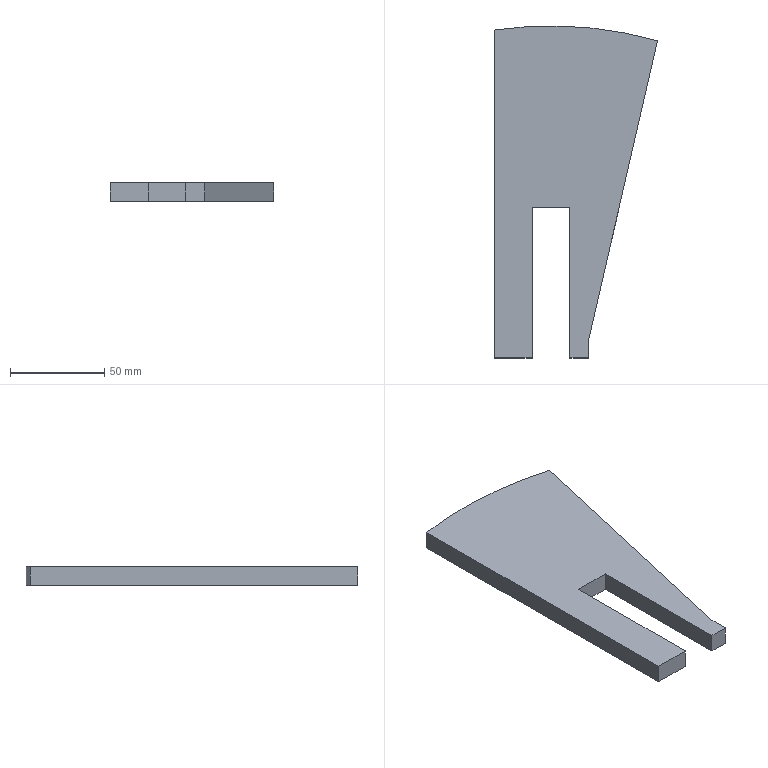Part | SolidWorks | features Extrusion 1, ICE 1 | 1 solid | 11 faces | box 86.5 x 176 x 10 mm | volume 102042 mm3 | plane 10 | cylinder 1 | commonest cylinder face diameters 412 x1
STEP:
#1=CARTESIAN_POINT('',(-30.,30.,-5.));
#2=VERTEX_POINT('',#1);
#3=CARTESIAN_POINT('',(-10.,30.,-5.));
#4=VERTEX_POINT('',#3);
#5=CARTESIAN_POINT('',(20.,30.,-5.));
#6=DIRECTION('',(1.,0.,0.));
#7=VECTOR('',#6,1000.);
#8=LINE('',#5,#7);
#9=EDGE_CURVE('',#2,#4,#8,.T.);
#10=ORIENTED_EDGE('',*,*,#9,.T.);
#11=CARTESIAN_POINT('',(-10.,30.,5.));
#12=VERTEX_POINT('',#11);
#13=CARTESIAN_POINT('',(-10.,30.,5.));
#14=DIRECTION('',(0.,0.,1.));
#15=VECTOR('',#14,1000.);
#16=LINE('',#13,#15);
#17=EDGE_CURVE('',#4,#12,#16,.T.);
#18=ORIENTED_EDGE('',*,*,#17,.T.);
#19=CARTESIAN_POINT('',(-30.,30.,5.));
#20=VERTEX_POINT('',#19);
#21=CARTESIAN_POINT('',(20.,30.,5.));
#22=DIRECTION('',(1.,0.,0.));
#23=VECTOR('',#22,1000.);
#24=LINE('',#21,#23);
#25=EDGE_CURVE('',#20,#12,#24,.T.);
#26=ORIENTED_EDGE('',*,*,#25,.F.);
#27=CARTESIAN_POINT('',(-30.,30.,5.));
#28=DIRECTION('',(0.,0.,-1.));
#29=VECTOR('',#28,1000.);
#30=LINE('',#27,#29);
#31=EDGE_CURVE('',#20,#2,#30,.T.);
#32=ORIENTED_EDGE('',*,*,#31,.T.);
#33=EDGE_LOOP('',(#10,#18,#26,#32));
#34=FACE_OUTER_BOUND('',#33,.T.);
#35=CARTESIAN_POINT('',(20.,30.,5.));
#36=DIRECTION('',(0.,1.,0.));
#37=DIRECTION('',(-1.,0.,0.));
#38=AXIS2_PLACEMENT_3D('',#35,#36,#37);
#39=PLANE('',#38);
#40=ADVANCED_FACE('',(#34),#39,.F.);
#41=CARTESIAN_POINT('',(56.5,198.1,-5.));
#42=VERTEX_POINT('',#41);
#43=CARTESIAN_POINT('',(-30.,203.804,-5.));
#44=VERTEX_POINT('',#43);
#45=CARTESIAN_POINT('',(0.,0.,-5.));
#46=DIRECTION('',(0.,0.,1.));
#47=DIRECTION('',(1.,0.,0.));
#48=AXIS2_PLACEMENT_3D('',#45,#46,#47);
#49=CIRCLE('',#48,206.);
#50=EDGE_CURVE('',#42,#44,#49,.T.);
#51=ORIENTED_EDGE('',*,*,#50,.T.);
#52=CARTESIAN_POINT('',(-30.,203.804,5.));
#53=VERTEX_POINT('',#52);
#54=CARTESIAN_POINT('',(-30.,203.804,5.));
#55=DIRECTION('',(0.,0.,-1.));
#56=VECTOR('',#55,1000.);
#57=LINE('',#54,#56);
#58=EDGE_CURVE('',#53,#44,#57,.T.);
#59=ORIENTED_EDGE('',*,*,#58,.F.);
#60=CARTESIAN_POINT('',(56.5,198.1,5.));
#61=VERTEX_POINT('',#60);
#62=CARTESIAN_POINT('',(0.,0.,5.));
#63=DIRECTION('',(0.,0.,1.));
#64=DIRECTION('',(1.,0.,0.));
#65=AXIS2_PLACEMENT_3D('',#62,#63,#64);
#66=CIRCLE('',#65,206.);
#67=EDGE_CURVE('',#61,#53,#66,.T.);
#68=ORIENTED_EDGE('',*,*,#67,.F.);
#69=CARTESIAN_POINT('',(56.5,198.1,5.));
#70=DIRECTION('',(0.,0.,-1.));
#71=VECTOR('',#70,1000.);
#72=LINE('',#69,#71);
#73=EDGE_CURVE('',#61,#42,#72,.T.);
#74=ORIENTED_EDGE('',*,*,#73,.T.);
#75=EDGE_LOOP('',(#51,#59,#68,#74));
#76=FACE_OUTER_BOUND('',#75,.T.);
#77=CARTESIAN_POINT('',(0.,0.,5.));
#78=DIRECTION('',(0.,0.,-1.));
#79=DIRECTION('',(-1.,0.,0.));
#80=AXIS2_PLACEMENT_3D('',#77,#78,#79);
#81=CYLINDRICAL_SURFACE('',#80,206.);
#82=ADVANCED_FACE('',(#76),#81,.T.);
#83=CARTESIAN_POINT('',(-30.,203.804,-5.));
#84=DIRECTION('',(0.,-1.,0.));
#85=VECTOR('',#84,1000.);
#86=LINE('',#83,#85);
#87=EDGE_CURVE('',#44,#2,#86,.T.);
#88=ORIENTED_EDGE('',*,*,#87,.T.);
#89=ORIENTED_EDGE('',*,*,#31,.F.);
#90=CARTESIAN_POINT('',(-30.,203.804,5.));
#91=DIRECTION('',(0.,-1.,0.));
#92=VECTOR('',#91,1000.);
#93=LINE('',#90,#92);
#94=EDGE_CURVE('',#53,#20,#93,.T.);
#95=ORIENTED_EDGE('',*,*,#94,.F.);
#96=ORIENTED_EDGE('',*,*,#58,.T.);
#97=EDGE_LOOP('',(#88,#89,#95,#96));
#98=FACE_OUTER_BOUND('',#97,.T.);
#99=CARTESIAN_POINT('',(-30.,203.804,5.));
#100=DIRECTION('',(1.,0.,0.));
#101=DIRECTION('',(0.,1.,0.));
#102=AXIS2_PLACEMENT_3D('',#99,#100,#101);
#103=PLANE('',#102);
#104=ADVANCED_FACE('',(#98),#103,.F.);
#105=CARTESIAN_POINT('',(10.,30.,5.));
#106=VERTEX_POINT('',#105);
#107=CARTESIAN_POINT('',(20.,30.,5.));
#108=VERTEX_POINT('',#107);
#109=CARTESIAN_POINT('',(20.,30.,5.));
#110=DIRECTION('',(1.,0.,0.));
#111=VECTOR('',#110,1000.);
#112=LINE('',#109,#111);
#113=EDGE_CURVE('',#106,#108,#112,.T.);
#114=ORIENTED_EDGE('',*,*,#113,.F.);
#115=CARTESIAN_POINT('',(10.,30.,-5.));
#116=VERTEX_POINT('',#115);
#117=CARTESIAN_POINT('',(10.,30.,5.));
#118=DIRECTION('',(0.,0.,-1.));
#119=VECTOR('',#118,1000.);
#120=LINE('',#117,#119);
#121=EDGE_CURVE('',#106,#116,#120,.T.);
#122=ORIENTED_EDGE('',*,*,#121,.T.);
#123=CARTESIAN_POINT('',(20.,30.,-5.));
#124=VERTEX_POINT('',#123);
#125=CARTESIAN_POINT('',(20.,30.,-5.));
#126=DIRECTION('',(1.,0.,0.));
#127=VECTOR('',#126,1000.);
#128=LINE('',#125,#127);
#129=EDGE_CURVE('',#116,#124,#128,.T.);
#130=ORIENTED_EDGE('',*,*,#129,.T.);
#131=CARTESIAN_POINT('',(20.,30.,5.));
#132=DIRECTION('',(0.,0.,-1.));
#133=VECTOR('',#132,1000.);
#134=LINE('',#131,#133);
#135=EDGE_CURVE('',#108,#124,#134,.T.);
#136=ORIENTED_EDGE('',*,*,#135,.F.);
#137=EDGE_LOOP('',(#114,#122,#130,#136));
#138=FACE_OUTER_BOUND('',#137,.T.);
#139=CARTESIAN_POINT('',(20.,30.,5.));
#140=DIRECTION('',(0.,1.,0.));
#141=DIRECTION('',(-1.,0.,0.));
#142=AXIS2_PLACEMENT_3D('',#139,#140,#141);
#143=PLANE('',#142);
#144=ADVANCED_FACE('',(#138),#143,.F.);
#145=CARTESIAN_POINT('',(20.,40.,-5.));
#146=VERTEX_POINT('',#145);
#147=CARTESIAN_POINT('',(20.,30.,-5.));
#148=DIRECTION('',(0.,1.,0.));
#149=VECTOR('',#148,1000.);
#150=LINE('',#147,#149);
#151=EDGE_CURVE('',#124,#146,#150,.T.);
#152=ORIENTED_EDGE('',*,*,#151,.T.);
#153=CARTESIAN_POINT('',(20.,40.,5.));
#154=VERTEX_POINT('',#153);
#155=CARTESIAN_POINT('',(20.,40.,5.));
#156=DIRECTION('',(0.,0.,-1.));
#157=VECTOR('',#156,1000.);
#158=LINE('',#155,#157);
#159=EDGE_CURVE('',#154,#146,#158,.T.);
#160=ORIENTED_EDGE('',*,*,#159,.F.);
#161=CARTESIAN_POINT('',(20.,30.,5.));
#162=DIRECTION('',(0.,1.,0.));
#163=VECTOR('',#162,1000.);
#164=LINE('',#161,#163);
#165=EDGE_CURVE('',#108,#154,#164,.T.);
#166=ORIENTED_EDGE('',*,*,#165,.F.);
#167=ORIENTED_EDGE('',*,*,#135,.T.);
#168=EDGE_LOOP('',(#152,#160,#166,#167));
#169=FACE_OUTER_BOUND('',#168,.T.);
#170=CARTESIAN_POINT('',(20.,30.,5.));
#171=DIRECTION('',(-1.,0.,0.));
#172=DIRECTION('',(0.,-1.,0.));
#173=AXIS2_PLACEMENT_3D('',#170,#171,#172);
#174=PLANE('',#173);
#175=ADVANCED_FACE('',(#169),#174,.F.);
#176=CARTESIAN_POINT('',(20.,40.,-5.));
#177=DIRECTION('',(0.225,0.9744,0.));
#178=VECTOR('',#177,1000.);
#179=LINE('',#176,#178);
#180=EDGE_CURVE('',#146,#42,#179,.T.);
#181=ORIENTED_EDGE('',*,*,#180,.T.);
#182=ORIENTED_EDGE('',*,*,#73,.F.);
#183=CARTESIAN_POINT('',(20.,40.,5.));
#184=DIRECTION('',(0.225,0.9744,0.));
#185=VECTOR('',#184,1000.);
#186=LINE('',#183,#185);
#187=EDGE_CURVE('',#154,#61,#186,.T.);
#188=ORIENTED_EDGE('',*,*,#187,.F.);
#189=ORIENTED_EDGE('',*,*,#159,.T.);
#190=EDGE_LOOP('',(#181,#182,#188,#189));
#191=FACE_OUTER_BOUND('',#190,.T.);
#192=CARTESIAN_POINT('',(20.,40.,5.));
#193=DIRECTION('',(-0.9744,0.225,0.));
#194=DIRECTION('',(-0.225,-0.9744,0.));
#195=AXIS2_PLACEMENT_3D('',#192,#193,#194);
#196=PLANE('',#195);
#197=ADVANCED_FACE('',(#191),#196,.F.);
#198=CARTESIAN_POINT('',(-10.,110.,5.));
#199=VERTEX_POINT('',#198);
#200=CARTESIAN_POINT('',(-10.,-50.,5.));
#201=DIRECTION('',(0.,-1.,0.));
#202=VECTOR('',#201,1000.);
#203=LINE('',#200,#202);
#204=EDGE_CURVE('',#199,#12,#203,.T.);
#205=ORIENTED_EDGE('',*,*,#204,.F.);
#206=CARTESIAN_POINT('',(10.,110.,5.));
#207=VERTEX_POINT('',#206);
#208=CARTESIAN_POINT('',(10.,110.,5.));
#209=DIRECTION('',(-1.,0.,0.));
#210=VECTOR('',#209,1000.);
#211=LINE('',#208,#210);
#212=EDGE_CURVE('',#207,#199,#211,.T.);
#213=ORIENTED_EDGE('',*,*,#212,.F.);
#214=CARTESIAN_POINT('',(10.,-50.,5.));
#215=DIRECTION('',(0.,1.,0.));
#216=VECTOR('',#215,1000.);
#217=LINE('',#214,#216);
#218=EDGE_CURVE('',#106,#207,#217,.T.);
#219=ORIENTED_EDGE('',*,*,#218,.F.);
#220=ORIENTED_EDGE('',*,*,#113,.T.);
#221=ORIENTED_EDGE('',*,*,#165,.T.);
#222=ORIENTED_EDGE('',*,*,#187,.T.);
#223=ORIENTED_EDGE('',*,*,#67,.T.);
#224=ORIENTED_EDGE('',*,*,#94,.T.);
#225=ORIENTED_EDGE('',*,*,#25,.T.);
#226=EDGE_LOOP('',(#205,#213,#219,#220,#221,#222,#223,#224,#225));
#227=FACE_OUTER_BOUND('',#226,.T.);
#228=CARTESIAN_POINT('',(0.,0.,5.));
#229=DIRECTION('',(0.,0.,1.));
#230=DIRECTION('',(1.,0.,0.));
#231=AXIS2_PLACEMENT_3D('',#228,#229,#230);
#232=PLANE('',#231);
#233=ADVANCED_FACE('',(#227),#232,.T.);
#234=CARTESIAN_POINT('',(10.,110.,-5.));
#235=VERTEX_POINT('',#234);
#236=CARTESIAN_POINT('',(-10.,110.,-5.));
#237=VERTEX_POINT('',#236);
#238=CARTESIAN_POINT('',(10.,110.,-5.));
#239=DIRECTION('',(-1.,0.,0.));
#240=VECTOR('',#239,1000.);
#241=LINE('',#238,#240);
#242=EDGE_CURVE('',#235,#237,#241,.T.);
#243=ORIENTED_EDGE('',*,*,#242,.T.);
#244=CARTESIAN_POINT('',(-10.,-50.,-5.));
#245=DIRECTION('',(0.,-1.,0.));
#246=VECTOR('',#245,1000.);
#247=LINE('',#244,#246);
#248=EDGE_CURVE('',#237,#4,#247,.T.);
#249=ORIENTED_EDGE('',*,*,#248,.T.);
#250=ORIENTED_EDGE('',*,*,#9,.F.);
#251=ORIENTED_EDGE('',*,*,#87,.F.);
#252=ORIENTED_EDGE('',*,*,#50,.F.);
#253=ORIENTED_EDGE('',*,*,#180,.F.);
#254=ORIENTED_EDGE('',*,*,#151,.F.);
#255=ORIENTED_EDGE('',*,*,#129,.F.);
#256=CARTESIAN_POINT('',(10.,0.,-5.));
#257=DIRECTION('',(0.,1.,0.));
#258=VECTOR('',#257,1000.);
#259=LINE('',#256,#258);
#260=EDGE_CURVE('',#116,#235,#259,.T.);
#261=ORIENTED_EDGE('',*,*,#260,.T.);
#262=EDGE_LOOP('',(#243,#249,#250,#251,#252,#253,#254,#255,#261));
#263=FACE_OUTER_BOUND('',#262,.T.);
#264=CARTESIAN_POINT('',(0.,0.,-5.));
#265=DIRECTION('',(0.,0.,1.));
#266=DIRECTION('',(1.,0.,0.));
#267=AXIS2_PLACEMENT_3D('',#264,#265,#266);
#268=PLANE('',#267);
#269=ADVANCED_FACE('',(#263),#268,.F.);
#270=ORIENTED_EDGE('',*,*,#248,.F.);
#271=CARTESIAN_POINT('',(-10.,110.,-5.));
#272=DIRECTION('',(0.,0.,1.));
#273=VECTOR('',#272,1000.);
#274=LINE('',#271,#273);
#275=EDGE_CURVE('',#237,#199,#274,.T.);
#276=ORIENTED_EDGE('',*,*,#275,.T.);
#277=ORIENTED_EDGE('',*,*,#204,.T.);
#278=ORIENTED_EDGE('',*,*,#17,.F.);
#279=EDGE_LOOP('',(#270,#276,#277,#278));
#280=FACE_OUTER_BOUND('',#279,.T.);
#281=CARTESIAN_POINT('',(-10.,-50.,-5.));
#282=DIRECTION('',(-1.,0.,0.));
#283=DIRECTION('',(0.,0.,1.));
#284=AXIS2_PLACEMENT_3D('',#281,#282,#283);
#285=PLANE('',#284);
#286=ADVANCED_FACE('',(#280),#285,.F.);
#287=ORIENTED_EDGE('',*,*,#218,.T.);
#288=CARTESIAN_POINT('',(10.,110.,-5.));
#289=DIRECTION('',(0.,0.,1.));
#290=VECTOR('',#289,1000.);
#291=LINE('',#288,#290);
#292=EDGE_CURVE('',#235,#207,#291,.T.);
#293=ORIENTED_EDGE('',*,*,#292,.F.);
#294=ORIENTED_EDGE('',*,*,#260,.F.);
#295=ORIENTED_EDGE('',*,*,#121,.F.);
#296=EDGE_LOOP('',(#287,#293,#294,#295));
#297=FACE_OUTER_BOUND('',#296,.T.);
#298=CARTESIAN_POINT('',(10.,-50.,-5.));
#299=DIRECTION('',(1.,0.,0.));
#300=DIRECTION('',(0.,0.,-1.));
#301=AXIS2_PLACEMENT_3D('',#298,#299,#300);
#302=PLANE('',#301);
#303=ADVANCED_FACE('',(#297),#302,.F.);
#304=ORIENTED_EDGE('',*,*,#212,.T.);
#305=ORIENTED_EDGE('',*,*,#275,.F.);
#306=ORIENTED_EDGE('',*,*,#242,.F.);
#307=ORIENTED_EDGE('',*,*,#292,.T.);
#308=EDGE_LOOP('',(#304,#305,#306,#307));
#309=FACE_OUTER_BOUND('',#308,.T.);
#310=CARTESIAN_POINT('',(10.,110.,-5.));
#311=DIRECTION('',(0.,1.,0.));
#312=DIRECTION('',(0.,0.,1.));
#313=AXIS2_PLACEMENT_3D('',#310,#311,#312);
#314=PLANE('',#313);
#315=ADVANCED_FACE('',(#309),#314,.F.);
#316=CLOSED_SHELL('',(#40,#82,#104,#144,#175,#197,#233,#269,#286,#303,#315));
#317=MANIFOLD_SOLID_BREP('',#316);
#318=CARTESIAN_POINT('',(0.,0.,0.));
#319=DIRECTION('',(0.,0.,1.));
#320=DIRECTION('',(1.,0.,0.));
#321=AXIS2_PLACEMENT_3D('',#318,#319,#320);
#322=(LENGTH_UNIT()NAMED_UNIT(*)SI_UNIT(.MILLI.,.METRE.));
#323=UNCERTAINTY_MEASURE_WITH_UNIT(LENGTH_MEASURE(0.00001),#322,'','');
#324=(NAMED_UNIT(*)PLANE_ANGLE_UNIT()SI_UNIT($,.RADIAN.));
#325=(NAMED_UNIT(*)SI_UNIT($,.STERADIAN.)SOLID_ANGLE_UNIT());
#326=(GEOMETRIC_REPRESENTATION_CONTEXT(3)GLOBAL_UNCERTAINTY_ASSIGNED_CONTEXT((#323))GLOBAL_UNIT_ASSIGNED_CONTEXT((#322,#324,#325))REPRESENTATION_CONTEXT('',''));
#327=ADVANCED_BREP_SHAPE_REPRESENTATION('',(#317,#321),#326);